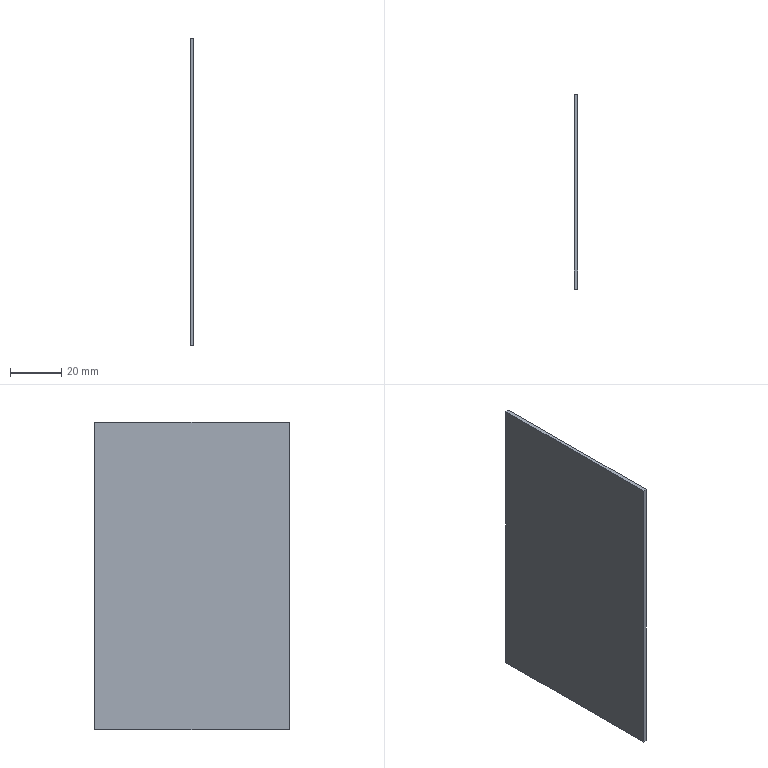Part | SolidWorks | features Extrusion 1 | 1 solid | 6 faces | box 1.5 x 76 x 120 mm | volume 13680 mm3 | plane 6
STEP:
#1=CARTESIAN_POINT('',(0.,-38.,-60.));
#2=VERTEX_POINT('',#1);
#3=CARTESIAN_POINT('',(0.,38.,-60.));
#4=VERTEX_POINT('',#3);
#5=CARTESIAN_POINT('',(0.,-38.,-60.));
#6=DIRECTION('',(0.,1.,0.));
#7=VECTOR('',#6,1000.);
#8=LINE('',#5,#7);
#9=EDGE_CURVE('',#2,#4,#8,.T.);
#10=ORIENTED_EDGE('',*,*,#9,.T.);
#11=CARTESIAN_POINT('',(1.5,38.,-60.));
#12=VERTEX_POINT('',#11);
#13=CARTESIAN_POINT('',(1.5,38.,-60.));
#14=DIRECTION('',(-1.,0.,0.));
#15=VECTOR('',#14,1000.);
#16=LINE('',#13,#15);
#17=EDGE_CURVE('',#12,#4,#16,.T.);
#18=ORIENTED_EDGE('',*,*,#17,.F.);
#19=CARTESIAN_POINT('',(1.5,-38.,-60.));
#20=VERTEX_POINT('',#19);
#21=CARTESIAN_POINT('',(1.5,-38.,-60.));
#22=DIRECTION('',(0.,1.,0.));
#23=VECTOR('',#22,1000.);
#24=LINE('',#21,#23);
#25=EDGE_CURVE('',#20,#12,#24,.T.);
#26=ORIENTED_EDGE('',*,*,#25,.F.);
#27=CARTESIAN_POINT('',(1.5,-38.,-60.));
#28=DIRECTION('',(-1.,0.,0.));
#29=VECTOR('',#28,1000.);
#30=LINE('',#27,#29);
#31=EDGE_CURVE('',#20,#2,#30,.T.);
#32=ORIENTED_EDGE('',*,*,#31,.T.);
#33=EDGE_LOOP('',(#10,#18,#26,#32));
#34=FACE_OUTER_BOUND('',#33,.T.);
#35=CARTESIAN_POINT('',(1.5,-38.,-60.));
#36=DIRECTION('',(0.,0.,1.));
#37=DIRECTION('',(1.,0.,0.));
#38=AXIS2_PLACEMENT_3D('',#35,#36,#37);
#39=PLANE('',#38);
#40=ADVANCED_FACE('',(#34),#39,.F.);
#41=CARTESIAN_POINT('',(0.,38.,60.));
#42=VERTEX_POINT('',#41);
#43=CARTESIAN_POINT('',(0.,38.,60.));
#44=DIRECTION('',(0.,0.,1.));
#45=VECTOR('',#44,1000.);
#46=LINE('',#43,#45);
#47=EDGE_CURVE('',#4,#42,#46,.T.);
#48=ORIENTED_EDGE('',*,*,#47,.T.);
#49=CARTESIAN_POINT('',(1.5,38.,60.));
#50=VERTEX_POINT('',#49);
#51=CARTESIAN_POINT('',(1.5,38.,60.));
#52=DIRECTION('',(-1.,0.,0.));
#53=VECTOR('',#52,1000.);
#54=LINE('',#51,#53);
#55=EDGE_CURVE('',#50,#42,#54,.T.);
#56=ORIENTED_EDGE('',*,*,#55,.F.);
#57=CARTESIAN_POINT('',(1.5,38.,60.));
#58=DIRECTION('',(0.,0.,1.));
#59=VECTOR('',#58,1000.);
#60=LINE('',#57,#59);
#61=EDGE_CURVE('',#12,#50,#60,.T.);
#62=ORIENTED_EDGE('',*,*,#61,.F.);
#63=ORIENTED_EDGE('',*,*,#17,.T.);
#64=EDGE_LOOP('',(#48,#56,#62,#63));
#65=FACE_OUTER_BOUND('',#64,.T.);
#66=CARTESIAN_POINT('',(1.5,38.,60.));
#67=DIRECTION('',(0.,-1.,0.));
#68=DIRECTION('',(0.,0.,-1.));
#69=AXIS2_PLACEMENT_3D('',#66,#67,#68);
#70=PLANE('',#69);
#71=ADVANCED_FACE('',(#65),#70,.F.);
#72=CARTESIAN_POINT('',(0.,-38.,60.));
#73=VERTEX_POINT('',#72);
#74=CARTESIAN_POINT('',(0.,-38.,60.));
#75=DIRECTION('',(0.,-1.,0.));
#76=VECTOR('',#75,1000.);
#77=LINE('',#74,#76);
#78=EDGE_CURVE('',#42,#73,#77,.T.);
#79=ORIENTED_EDGE('',*,*,#78,.T.);
#80=CARTESIAN_POINT('',(1.5,-38.,60.));
#81=VERTEX_POINT('',#80);
#82=CARTESIAN_POINT('',(1.5,-38.,60.));
#83=DIRECTION('',(-1.,0.,0.));
#84=VECTOR('',#83,1000.);
#85=LINE('',#82,#84);
#86=EDGE_CURVE('',#81,#73,#85,.T.);
#87=ORIENTED_EDGE('',*,*,#86,.F.);
#88=CARTESIAN_POINT('',(1.5,-38.,60.));
#89=DIRECTION('',(0.,-1.,0.));
#90=VECTOR('',#89,1000.);
#91=LINE('',#88,#90);
#92=EDGE_CURVE('',#50,#81,#91,.T.);
#93=ORIENTED_EDGE('',*,*,#92,.F.);
#94=ORIENTED_EDGE('',*,*,#55,.T.);
#95=EDGE_LOOP('',(#79,#87,#93,#94));
#96=FACE_OUTER_BOUND('',#95,.T.);
#97=CARTESIAN_POINT('',(1.5,-38.,60.));
#98=DIRECTION('',(0.,0.,-1.));
#99=DIRECTION('',(-1.,0.,0.));
#100=AXIS2_PLACEMENT_3D('',#97,#98,#99);
#101=PLANE('',#100);
#102=ADVANCED_FACE('',(#96),#101,.F.);
#103=CARTESIAN_POINT('',(0.,-38.,60.));
#104=DIRECTION('',(0.,0.,-1.));
#105=VECTOR('',#104,1000.);
#106=LINE('',#103,#105);
#107=EDGE_CURVE('',#73,#2,#106,.T.);
#108=ORIENTED_EDGE('',*,*,#107,.T.);
#109=ORIENTED_EDGE('',*,*,#31,.F.);
#110=CARTESIAN_POINT('',(1.5,-38.,60.));
#111=DIRECTION('',(0.,0.,-1.));
#112=VECTOR('',#111,1000.);
#113=LINE('',#110,#112);
#114=EDGE_CURVE('',#81,#20,#113,.T.);
#115=ORIENTED_EDGE('',*,*,#114,.F.);
#116=ORIENTED_EDGE('',*,*,#86,.T.);
#117=EDGE_LOOP('',(#108,#109,#115,#116));
#118=FACE_OUTER_BOUND('',#117,.T.);
#119=CARTESIAN_POINT('',(1.5,-38.,60.));
#120=DIRECTION('',(0.,1.,0.));
#121=DIRECTION('',(0.,0.,1.));
#122=AXIS2_PLACEMENT_3D('',#119,#120,#121);
#123=PLANE('',#122);
#124=ADVANCED_FACE('',(#118),#123,.F.);
#125=ORIENTED_EDGE('',*,*,#25,.T.);
#126=ORIENTED_EDGE('',*,*,#61,.T.);
#127=ORIENTED_EDGE('',*,*,#92,.T.);
#128=ORIENTED_EDGE('',*,*,#114,.T.);
#129=EDGE_LOOP('',(#125,#126,#127,#128));
#130=FACE_OUTER_BOUND('',#129,.T.);
#131=CARTESIAN_POINT('',(1.5,38.,-60.));
#132=DIRECTION('',(-1.,0.,0.));
#133=DIRECTION('',(0.,0.,1.));
#134=AXIS2_PLACEMENT_3D('',#131,#132,#133);
#135=PLANE('',#134);
#136=ADVANCED_FACE('',(#130),#135,.F.);
#137=ORIENTED_EDGE('',*,*,#9,.F.);
#138=ORIENTED_EDGE('',*,*,#107,.F.);
#139=ORIENTED_EDGE('',*,*,#78,.F.);
#140=ORIENTED_EDGE('',*,*,#47,.F.);
#141=EDGE_LOOP('',(#137,#138,#139,#140));
#142=FACE_OUTER_BOUND('',#141,.T.);
#143=CARTESIAN_POINT('',(0.,38.,-60.));
#144=DIRECTION('',(-1.,0.,0.));
#145=DIRECTION('',(0.,0.,1.));
#146=AXIS2_PLACEMENT_3D('',#143,#144,#145);
#147=PLANE('',#146);
#148=ADVANCED_FACE('',(#142),#147,.T.);
#149=CLOSED_SHELL('',(#40,#71,#102,#124,#136,#148));
#150=MANIFOLD_SOLID_BREP('',#149);
#151=CARTESIAN_POINT('',(0.,0.,0.));
#152=DIRECTION('',(0.,0.,1.));
#153=DIRECTION('',(1.,0.,0.));
#154=AXIS2_PLACEMENT_3D('',#151,#152,#153);
#155=(LENGTH_UNIT()NAMED_UNIT(*)SI_UNIT(.MILLI.,.METRE.));
#156=UNCERTAINTY_MEASURE_WITH_UNIT(LENGTH_MEASURE(0.00001),#155,'','');
#157=(NAMED_UNIT(*)PLANE_ANGLE_UNIT()SI_UNIT($,.RADIAN.));
#158=(NAMED_UNIT(*)SI_UNIT($,.STERADIAN.)SOLID_ANGLE_UNIT());
#159=(GEOMETRIC_REPRESENTATION_CONTEXT(3)GLOBAL_UNCERTAINTY_ASSIGNED_CONTEXT((#156))GLOBAL_UNIT_ASSIGNED_CONTEXT((#155,#157,#158))REPRESENTATION_CONTEXT('',''));
#160=ADVANCED_BREP_SHAPE_REPRESENTATION('',(#150,#154),#159);